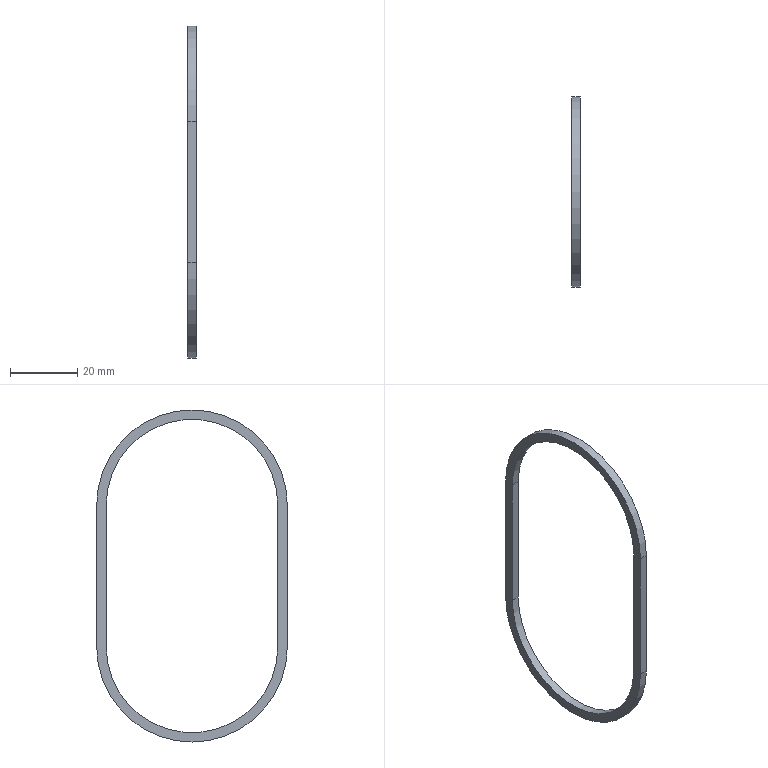Part | NX | features DATUM_CSYS 2, DATUM_PLANE 1, EXTRUDE 1, SKETCH 1 | 1 solid | 10 faces | box 2.5 x 56.6 x 98.6 mm | volume 1771 mm3 | plane 6 | cylinder 4 | commonest cylinder face diameters 51 x2 56.6 x2
STEP:
#1=CARTESIAN_POINT('',(0.,-25.5,-21.));
#2=VERTEX_POINT('',#1);
#3=CARTESIAN_POINT('',(0.,25.5,-21.));
#4=VERTEX_POINT('',#3);
#5=CARTESIAN_POINT('',(0.,0.,-21.));
#6=DIRECTION('',(1.,0.,0.));
#7=DIRECTION('',(0.,1.,0.));
#8=AXIS2_PLACEMENT_3D('',#5,#6,#7);
#9=CIRCLE('',#8,25.5);
#10=EDGE_CURVE('',#2,#4,#9,.T.);
#11=ORIENTED_EDGE('',*,*,#10,.F.);
#12=CARTESIAN_POINT('',(2.5,-25.5,-21.));
#13=VERTEX_POINT('',#12);
#14=CARTESIAN_POINT('',(2.5,-25.5,-21.));
#15=DIRECTION('',(-1.,0.,0.));
#16=VECTOR('',#15,1000.);
#17=LINE('',#14,#16);
#18=EDGE_CURVE('',#13,#2,#17,.T.);
#19=ORIENTED_EDGE('',*,*,#18,.F.);
#20=CARTESIAN_POINT('',(2.5,25.5,-21.));
#21=VERTEX_POINT('',#20);
#22=CARTESIAN_POINT('',(2.5,0.,-21.));
#23=DIRECTION('',(1.,0.,0.));
#24=DIRECTION('',(0.,1.,0.));
#25=AXIS2_PLACEMENT_3D('',#22,#23,#24);
#26=CIRCLE('',#25,25.5);
#27=EDGE_CURVE('',#13,#21,#26,.T.);
#28=ORIENTED_EDGE('',*,*,#27,.T.);
#29=CARTESIAN_POINT('',(2.5,25.5,-21.));
#30=DIRECTION('',(-1.,0.,0.));
#31=VECTOR('',#30,1000.);
#32=LINE('',#29,#31);
#33=EDGE_CURVE('',#21,#4,#32,.T.);
#34=ORIENTED_EDGE('',*,*,#33,.T.);
#35=EDGE_LOOP('',(#11,#19,#28,#34));
#36=FACE_BOUND('',#35,.T.);
#37=CARTESIAN_POINT('',(2.5,0.,-21.));
#38=DIRECTION('',(-1.,0.,0.));
#39=DIRECTION('',(0.,0.,1.));
#40=AXIS2_PLACEMENT_3D('',#37,#38,#39);
#41=CYLINDRICAL_SURFACE('',#40,25.5);
#42=ADVANCED_FACE('',(#36),#41,.F.);
#43=CARTESIAN_POINT('',(0.,-25.5,21.));
#44=VERTEX_POINT('',#43);
#45=CARTESIAN_POINT('',(0.,-25.5,21.));
#46=DIRECTION('',(0.,0.,-1.));
#47=VECTOR('',#46,1000.);
#48=LINE('',#45,#47);
#49=EDGE_CURVE('',#44,#2,#48,.T.);
#50=ORIENTED_EDGE('',*,*,#49,.F.);
#51=CARTESIAN_POINT('',(2.5,-25.5,21.));
#52=VERTEX_POINT('',#51);
#53=CARTESIAN_POINT('',(2.5,-25.5,21.));
#54=DIRECTION('',(-1.,0.,0.));
#55=VECTOR('',#54,1000.);
#56=LINE('',#53,#55);
#57=EDGE_CURVE('',#52,#44,#56,.T.);
#58=ORIENTED_EDGE('',*,*,#57,.F.);
#59=CARTESIAN_POINT('',(2.5,-25.5,21.));
#60=DIRECTION('',(0.,0.,-1.));
#61=VECTOR('',#60,1000.);
#62=LINE('',#59,#61);
#63=EDGE_CURVE('',#52,#13,#62,.T.);
#64=ORIENTED_EDGE('',*,*,#63,.T.);
#65=ORIENTED_EDGE('',*,*,#18,.T.);
#66=EDGE_LOOP('',(#50,#58,#64,#65));
#67=FACE_BOUND('',#66,.T.);
#68=CARTESIAN_POINT('',(2.5,-25.5,21.));
#69=DIRECTION('',(0.,1.,0.));
#70=DIRECTION('',(0.,0.,1.));
#71=AXIS2_PLACEMENT_3D('',#68,#69,#70);
#72=PLANE('',#71);
#73=ADVANCED_FACE('',(#67),#72,.T.);
#74=CARTESIAN_POINT('',(0.,25.5,21.));
#75=VERTEX_POINT('',#74);
#76=CARTESIAN_POINT('',(0.,0.,21.));
#77=DIRECTION('',(1.,0.,0.));
#78=DIRECTION('',(0.,1.,0.));
#79=AXIS2_PLACEMENT_3D('',#76,#77,#78);
#80=CIRCLE('',#79,25.5);
#81=EDGE_CURVE('',#75,#44,#80,.T.);
#82=ORIENTED_EDGE('',*,*,#81,.F.);
#83=CARTESIAN_POINT('',(2.5,25.5,21.));
#84=VERTEX_POINT('',#83);
#85=CARTESIAN_POINT('',(2.5,25.5,21.));
#86=DIRECTION('',(-1.,0.,0.));
#87=VECTOR('',#86,1000.);
#88=LINE('',#85,#87);
#89=EDGE_CURVE('',#84,#75,#88,.T.);
#90=ORIENTED_EDGE('',*,*,#89,.F.);
#91=CARTESIAN_POINT('',(2.5,0.,21.));
#92=DIRECTION('',(1.,0.,0.));
#93=DIRECTION('',(0.,1.,0.));
#94=AXIS2_PLACEMENT_3D('',#91,#92,#93);
#95=CIRCLE('',#94,25.5);
#96=EDGE_CURVE('',#84,#52,#95,.T.);
#97=ORIENTED_EDGE('',*,*,#96,.T.);
#98=ORIENTED_EDGE('',*,*,#57,.T.);
#99=EDGE_LOOP('',(#82,#90,#97,#98));
#100=FACE_BOUND('',#99,.T.);
#101=CARTESIAN_POINT('',(2.5,0.,21.));
#102=DIRECTION('',(-1.,0.,0.));
#103=DIRECTION('',(0.,0.,1.));
#104=AXIS2_PLACEMENT_3D('',#101,#102,#103);
#105=CYLINDRICAL_SURFACE('',#104,25.5);
#106=ADVANCED_FACE('',(#100),#105,.F.);
#107=CARTESIAN_POINT('',(0.,28.3,21.));
#108=VERTEX_POINT('',#107);
#109=CARTESIAN_POINT('',(0.,-28.3,21.));
#110=VERTEX_POINT('',#109);
#111=CARTESIAN_POINT('',(0.,0.,21.));
#112=DIRECTION('',(1.,0.,0.));
#113=DIRECTION('',(0.,1.,0.));
#114=AXIS2_PLACEMENT_3D('',#111,#112,#113);
#115=CIRCLE('',#114,28.3);
#116=EDGE_CURVE('',#108,#110,#115,.T.);
#117=ORIENTED_EDGE('',*,*,#116,.T.);
#118=CARTESIAN_POINT('',(2.5,-28.3,21.));
#119=VERTEX_POINT('',#118);
#120=CARTESIAN_POINT('',(2.5,-28.3,21.));
#121=DIRECTION('',(-1.,0.,0.));
#122=VECTOR('',#121,1000.);
#123=LINE('',#120,#122);
#124=EDGE_CURVE('',#119,#110,#123,.T.);
#125=ORIENTED_EDGE('',*,*,#124,.F.);
#126=CARTESIAN_POINT('',(2.5,28.3,21.));
#127=VERTEX_POINT('',#126);
#128=CARTESIAN_POINT('',(2.5,0.,21.));
#129=DIRECTION('',(1.,0.,0.));
#130=DIRECTION('',(0.,1.,0.));
#131=AXIS2_PLACEMENT_3D('',#128,#129,#130);
#132=CIRCLE('',#131,28.3);
#133=EDGE_CURVE('',#127,#119,#132,.T.);
#134=ORIENTED_EDGE('',*,*,#133,.F.);
#135=CARTESIAN_POINT('',(2.5,28.3,21.));
#136=DIRECTION('',(-1.,0.,0.));
#137=VECTOR('',#136,1000.);
#138=LINE('',#135,#137);
#139=EDGE_CURVE('',#127,#108,#138,.T.);
#140=ORIENTED_EDGE('',*,*,#139,.T.);
#141=EDGE_LOOP('',(#117,#125,#134,#140));
#142=FACE_BOUND('',#141,.T.);
#143=CARTESIAN_POINT('',(2.5,0.,21.));
#144=DIRECTION('',(-1.,0.,0.));
#145=DIRECTION('',(0.,0.,1.));
#146=AXIS2_PLACEMENT_3D('',#143,#144,#145);
#147=CYLINDRICAL_SURFACE('',#146,28.3);
#148=ADVANCED_FACE('',(#142),#147,.T.);
#149=CARTESIAN_POINT('',(0.,-28.3,-21.));
#150=VERTEX_POINT('',#149);
#151=CARTESIAN_POINT('',(0.,-28.3,21.));
#152=DIRECTION('',(0.,0.,-1.));
#153=VECTOR('',#152,1000.);
#154=LINE('',#151,#153);
#155=EDGE_CURVE('',#110,#150,#154,.T.);
#156=ORIENTED_EDGE('',*,*,#155,.T.);
#157=CARTESIAN_POINT('',(2.5,-28.3,-21.));
#158=VERTEX_POINT('',#157);
#159=CARTESIAN_POINT('',(2.5,-28.3,-21.));
#160=DIRECTION('',(-1.,0.,0.));
#161=VECTOR('',#160,1000.);
#162=LINE('',#159,#161);
#163=EDGE_CURVE('',#158,#150,#162,.T.);
#164=ORIENTED_EDGE('',*,*,#163,.F.);
#165=CARTESIAN_POINT('',(2.5,-28.3,21.));
#166=DIRECTION('',(0.,0.,-1.));
#167=VECTOR('',#166,1000.);
#168=LINE('',#165,#167);
#169=EDGE_CURVE('',#119,#158,#168,.T.);
#170=ORIENTED_EDGE('',*,*,#169,.F.);
#171=ORIENTED_EDGE('',*,*,#124,.T.);
#172=EDGE_LOOP('',(#156,#164,#170,#171));
#173=FACE_BOUND('',#172,.T.);
#174=CARTESIAN_POINT('',(2.5,-28.3,21.));
#175=DIRECTION('',(0.,1.,0.));
#176=DIRECTION('',(0.,0.,1.));
#177=AXIS2_PLACEMENT_3D('',#174,#175,#176);
#178=PLANE('',#177);
#179=ADVANCED_FACE('',(#173),#178,.F.);
#180=CARTESIAN_POINT('',(0.,28.3,-21.));
#181=VERTEX_POINT('',#180);
#182=CARTESIAN_POINT('',(0.,0.,-21.));
#183=DIRECTION('',(1.,0.,0.));
#184=DIRECTION('',(0.,1.,0.));
#185=AXIS2_PLACEMENT_3D('',#182,#183,#184);
#186=CIRCLE('',#185,28.3);
#187=EDGE_CURVE('',#150,#181,#186,.T.);
#188=ORIENTED_EDGE('',*,*,#187,.T.);
#189=CARTESIAN_POINT('',(2.5,28.3,-21.));
#190=VERTEX_POINT('',#189);
#191=CARTESIAN_POINT('',(2.5,28.3,-21.));
#192=DIRECTION('',(-1.,0.,0.));
#193=VECTOR('',#192,1000.);
#194=LINE('',#191,#193);
#195=EDGE_CURVE('',#190,#181,#194,.T.);
#196=ORIENTED_EDGE('',*,*,#195,.F.);
#197=CARTESIAN_POINT('',(2.5,0.,-21.));
#198=DIRECTION('',(1.,0.,0.));
#199=DIRECTION('',(0.,1.,0.));
#200=AXIS2_PLACEMENT_3D('',#197,#198,#199);
#201=CIRCLE('',#200,28.3);
#202=EDGE_CURVE('',#158,#190,#201,.T.);
#203=ORIENTED_EDGE('',*,*,#202,.F.);
#204=ORIENTED_EDGE('',*,*,#163,.T.);
#205=EDGE_LOOP('',(#188,#196,#203,#204));
#206=FACE_BOUND('',#205,.T.);
#207=CARTESIAN_POINT('',(2.5,0.,-21.));
#208=DIRECTION('',(-1.,0.,0.));
#209=DIRECTION('',(0.,0.,1.));
#210=AXIS2_PLACEMENT_3D('',#207,#208,#209);
#211=CYLINDRICAL_SURFACE('',#210,28.3);
#212=ADVANCED_FACE('',(#206),#211,.T.);
#213=CARTESIAN_POINT('',(0.,28.3,-21.));
#214=DIRECTION('',(0.,0.,1.));
#215=VECTOR('',#214,1000.);
#216=LINE('',#213,#215);
#217=EDGE_CURVE('',#181,#108,#216,.T.);
#218=ORIENTED_EDGE('',*,*,#217,.T.);
#219=ORIENTED_EDGE('',*,*,#139,.F.);
#220=CARTESIAN_POINT('',(2.5,28.3,-21.));
#221=DIRECTION('',(0.,0.,1.));
#222=VECTOR('',#221,1000.);
#223=LINE('',#220,#222);
#224=EDGE_CURVE('',#190,#127,#223,.T.);
#225=ORIENTED_EDGE('',*,*,#224,.F.);
#226=ORIENTED_EDGE('',*,*,#195,.T.);
#227=EDGE_LOOP('',(#218,#219,#225,#226));
#228=FACE_BOUND('',#227,.T.);
#229=CARTESIAN_POINT('',(2.5,28.3,-21.));
#230=DIRECTION('',(0.,-1.,0.));
#231=DIRECTION('',(0.,0.,-1.));
#232=AXIS2_PLACEMENT_3D('',#229,#230,#231);
#233=PLANE('',#232);
#234=ADVANCED_FACE('',(#228),#233,.F.);
#235=CARTESIAN_POINT('',(0.,25.5,-21.));
#236=DIRECTION('',(0.,0.,1.));
#237=VECTOR('',#236,1000.);
#238=LINE('',#235,#237);
#239=EDGE_CURVE('',#4,#75,#238,.T.);
#240=ORIENTED_EDGE('',*,*,#239,.F.);
#241=ORIENTED_EDGE('',*,*,#33,.F.);
#242=CARTESIAN_POINT('',(2.5,25.5,-21.));
#243=DIRECTION('',(0.,0.,1.));
#244=VECTOR('',#243,1000.);
#245=LINE('',#242,#244);
#246=EDGE_CURVE('',#21,#84,#245,.T.);
#247=ORIENTED_EDGE('',*,*,#246,.T.);
#248=ORIENTED_EDGE('',*,*,#89,.T.);
#249=EDGE_LOOP('',(#240,#241,#247,#248));
#250=FACE_BOUND('',#249,.T.);
#251=CARTESIAN_POINT('',(2.5,25.5,-21.));
#252=DIRECTION('',(0.,-1.,0.));
#253=DIRECTION('',(0.,0.,-1.));
#254=AXIS2_PLACEMENT_3D('',#251,#252,#253);
#255=PLANE('',#254);
#256=ADVANCED_FACE('',(#250),#255,.T.);
#257=ORIENTED_EDGE('',*,*,#133,.T.);
#258=ORIENTED_EDGE('',*,*,#169,.T.);
#259=ORIENTED_EDGE('',*,*,#202,.T.);
#260=ORIENTED_EDGE('',*,*,#224,.T.);
#261=EDGE_LOOP('',(#257,#258,#259,#260));
#262=FACE_BOUND('',#261,.T.);
#263=ORIENTED_EDGE('',*,*,#27,.F.);
#264=ORIENTED_EDGE('',*,*,#63,.F.);
#265=ORIENTED_EDGE('',*,*,#96,.F.);
#266=ORIENTED_EDGE('',*,*,#246,.F.);
#267=EDGE_LOOP('',(#263,#264,#265,#266));
#268=FACE_BOUND('',#267,.T.);
#269=CARTESIAN_POINT('',(2.5,0.,21.));
#270=DIRECTION('',(1.,0.,0.));
#271=DIRECTION('',(0.,0.,-1.));
#272=AXIS2_PLACEMENT_3D('',#269,#270,#271);
#273=PLANE('',#272);
#274=ADVANCED_FACE('',(#262,#268),#273,.T.);
#275=ORIENTED_EDGE('',*,*,#116,.F.);
#276=ORIENTED_EDGE('',*,*,#217,.F.);
#277=ORIENTED_EDGE('',*,*,#187,.F.);
#278=ORIENTED_EDGE('',*,*,#155,.F.);
#279=EDGE_LOOP('',(#275,#276,#277,#278));
#280=FACE_BOUND('',#279,.T.);
#281=ORIENTED_EDGE('',*,*,#10,.T.);
#282=ORIENTED_EDGE('',*,*,#239,.T.);
#283=ORIENTED_EDGE('',*,*,#81,.T.);
#284=ORIENTED_EDGE('',*,*,#49,.T.);
#285=EDGE_LOOP('',(#281,#282,#283,#284));
#286=FACE_BOUND('',#285,.T.);
#287=CARTESIAN_POINT('',(0.,0.,21.));
#288=DIRECTION('',(1.,0.,0.));
#289=DIRECTION('',(0.,0.,-1.));
#290=AXIS2_PLACEMENT_3D('',#287,#288,#289);
#291=PLANE('',#290);
#292=ADVANCED_FACE('',(#280,#286),#291,.F.);
#293=CLOSED_SHELL('',(#42,#73,#106,#148,#179,#212,#234,#256,#274,#292));
#294=MANIFOLD_SOLID_BREP('',#293);
#295=(LENGTH_UNIT()NAMED_UNIT(*)SI_UNIT(.MILLI.,.METRE.));
#296=UNCERTAINTY_MEASURE_WITH_UNIT(LENGTH_MEASURE(0.00001),#295,'','');
#297=(NAMED_UNIT(*)PLANE_ANGLE_UNIT()SI_UNIT($,.RADIAN.));
#298=(NAMED_UNIT(*)SI_UNIT($,.STERADIAN.)SOLID_ANGLE_UNIT());
#299=(GEOMETRIC_REPRESENTATION_CONTEXT(3)GLOBAL_UNCERTAINTY_ASSIGNED_CONTEXT((#296))GLOBAL_UNIT_ASSIGNED_CONTEXT((#295,#297,#298))REPRESENTATION_CONTEXT('',''));
#300=ADVANCED_BREP_SHAPE_REPRESENTATION('',(#294),#299);